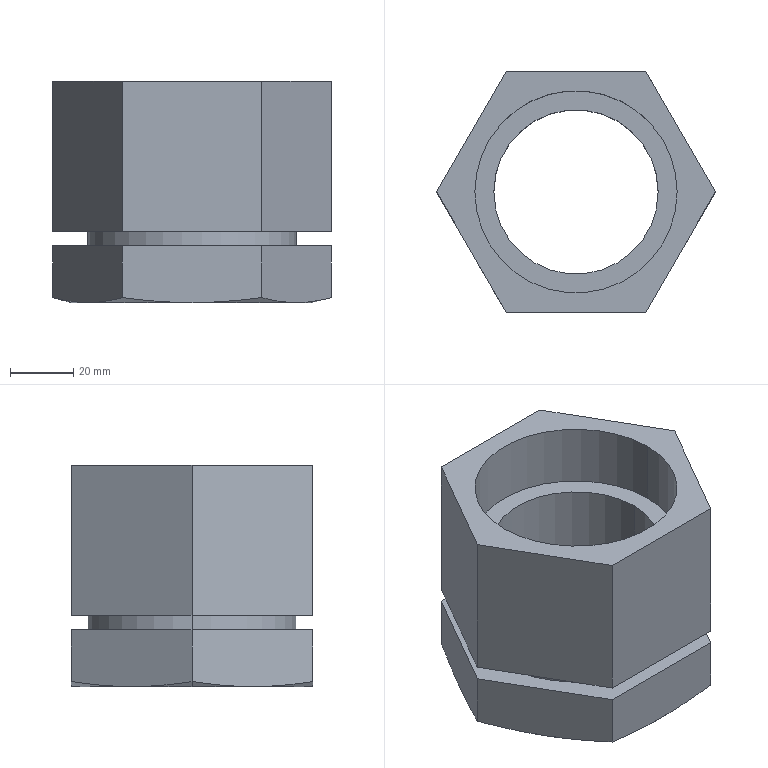Part | NX | features BREP 1 | 1 solid | 30 faces | box 88.25 x 76.427 x 70 mm | volume 175970 mm3 | plane 17 | cone 7 | cylinder 6 | commonest cylinder face diameters 52 x2 64 x2 66 x2
STEP:
#1=CARTESIAN_POINT('',(-33.,0.,22.5));
#2=VERTEX_POINT('',#1);
#3=CARTESIAN_POINT('',(33.,0.,22.5));
#4=VERTEX_POINT('',#3);
#5=CARTESIAN_POINT('',(0.,0.,22.5));
#6=DIRECTION('',(0.,0.,-1.));
#7=DIRECTION('',(-1.,0.,0.));
#8=AXIS2_PLACEMENT_3D('',#5,#6,#7);
#9=CIRCLE('',#8,33.);
#10=EDGE_CURVE('',#2,#4,#9,.T.);
#11=ORIENTED_EDGE('',*,*,#10,.T.);
#12=CARTESIAN_POINT('',(33.,0.,18.));
#13=VERTEX_POINT('',#12);
#14=CARTESIAN_POINT('',(33.,0.,0.));
#15=DIRECTION('',(0.,0.,-1.));
#16=VECTOR('',#15,1000.);
#17=LINE('',#14,#16);
#18=EDGE_CURVE('',#13,#4,#17,.F.);
#19=ORIENTED_EDGE('',*,*,#18,.F.);
#20=CARTESIAN_POINT('',(-33.,0.,18.));
#21=VERTEX_POINT('',#20);
#22=CARTESIAN_POINT('',(0.,0.,18.));
#23=DIRECTION('',(0.,0.,-1.));
#24=DIRECTION('',(-1.,0.,0.));
#25=AXIS2_PLACEMENT_3D('',#22,#23,#24);
#26=CIRCLE('',#25,33.);
#27=EDGE_CURVE('',#21,#13,#26,.T.);
#28=ORIENTED_EDGE('',*,*,#27,.F.);
#29=CARTESIAN_POINT('',(-33.,0.,0.));
#30=DIRECTION('',(0.,0.,-1.));
#31=VECTOR('',#30,1000.);
#32=LINE('',#29,#31);
#33=EDGE_CURVE('',#21,#2,#32,.F.);
#34=ORIENTED_EDGE('',*,*,#33,.T.);
#35=EDGE_LOOP('',(#11,#19,#28,#34));
#36=FACE_BOUND('',#35,.T.);
#37=CARTESIAN_POINT('',(0.,0.,0.));
#38=DIRECTION('',(0.,0.,-1.));
#39=DIRECTION('',(1.,0.,0.));
#40=AXIS2_PLACEMENT_3D('',#37,#38,#39);
#41=CYLINDRICAL_SURFACE('',#40,33.);
#42=ADVANCED_FACE('',(#36),#41,.T.);
#43=CARTESIAN_POINT('',(-32.,0.,70.));
#44=VERTEX_POINT('',#43);
#45=CARTESIAN_POINT('',(32.,0.,70.));
#46=VERTEX_POINT('',#45);
#47=CARTESIAN_POINT('',(0.,0.,70.));
#48=DIRECTION('',(0.,0.,1.));
#49=DIRECTION('',(1.,0.,0.));
#50=AXIS2_PLACEMENT_3D('',#47,#48,#49);
#51=CIRCLE('',#50,32.);
#52=EDGE_CURVE('',#44,#46,#51,.T.);
#53=ORIENTED_EDGE('',*,*,#52,.T.);
#54=CARTESIAN_POINT('',(32.,0.,50.));
#55=VERTEX_POINT('',#54);
#56=CARTESIAN_POINT('',(32.,0.,70.));
#57=DIRECTION('',(0.,0.,-1.));
#58=VECTOR('',#57,1000.);
#59=LINE('',#56,#58);
#60=EDGE_CURVE('',#55,#46,#59,.F.);
#61=ORIENTED_EDGE('',*,*,#60,.F.);
#62=CARTESIAN_POINT('',(-32.,0.,50.));
#63=VERTEX_POINT('',#62);
#64=CARTESIAN_POINT('',(0.,0.,50.));
#65=DIRECTION('',(0.,0.,1.));
#66=DIRECTION('',(1.,0.,0.));
#67=AXIS2_PLACEMENT_3D('',#64,#65,#66);
#68=CIRCLE('',#67,32.);
#69=EDGE_CURVE('',#63,#55,#68,.T.);
#70=ORIENTED_EDGE('',*,*,#69,.F.);
#71=CARTESIAN_POINT('',(-32.,0.,70.));
#72=DIRECTION('',(0.,0.,-1.));
#73=VECTOR('',#72,1000.);
#74=LINE('',#71,#73);
#75=EDGE_CURVE('',#63,#44,#74,.F.);
#76=ORIENTED_EDGE('',*,*,#75,.T.);
#77=EDGE_LOOP('',(#53,#61,#70,#76));
#78=FACE_BOUND('',#77,.T.);
#79=CARTESIAN_POINT('',(0.,0.,70.));
#80=DIRECTION('',(0.,0.,-1.));
#81=DIRECTION('',(1.,0.,0.));
#82=AXIS2_PLACEMENT_3D('',#79,#80,#81);
#83=CYLINDRICAL_SURFACE('',#82,32.);
#84=ADVANCED_FACE('',(#78),#83,.F.);
#85=CARTESIAN_POINT('',(-38.213,0.,0.));
#86=VERTEX_POINT('',#85);
#87=CARTESIAN_POINT('',(-33.094,19.107,0.));
#88=VERTEX_POINT('',#87);
#89=CARTESIAN_POINT('',(0.,0.,0.));
#90=DIRECTION('',(0.,0.,-1.));
#91=DIRECTION('',(-1.,0.,0.));
#92=AXIS2_PLACEMENT_3D('',#89,#90,#91);
#93=CIRCLE('',#92,38.213);
#94=EDGE_CURVE('',#86,#88,#93,.T.);
#95=ORIENTED_EDGE('',*,*,#94,.F.);
#96=CARTESIAN_POINT('',(-44.125,0.,1.584));
#97=VERTEX_POINT('',#96);
#98=CARTESIAN_POINT('',(-38.213,0.,0.));
#99=DIRECTION('',(-0.9659,0.,0.2588));
#100=VECTOR('',#99,1000.);
#101=LINE('',#98,#100);
#102=EDGE_CURVE('',#86,#97,#101,.T.);
#103=ORIENTED_EDGE('',*,*,#102,.T.);
#104=CARTESIAN_POINT('',(-44.125,0.,1.584));
#105=CARTESIAN_POINT('',(-40.464,6.341,0.6031));
#106=CARTESIAN_POINT('',(-36.79,12.705,0.));
#107=CARTESIAN_POINT('',(-33.094,19.107,0.));
#108=B_SPLINE_CURVE_WITH_KNOTS('',3,(#104,#105,#106,#107),.UNSPECIFIED.,.F.,.F.,(4,4),(0.,0.02212),.UNSPECIFIED.);
#109=EDGE_CURVE('',#97,#88,#108,.T.);
#110=ORIENTED_EDGE('',*,*,#109,.T.);
#111=EDGE_LOOP('',(#95,#103,#110));
#112=FACE_BOUND('',#111,.T.);
#113=CARTESIAN_POINT('',(0.,0.,0.));
#114=DIRECTION('',(0.,0.,1.));
#115=DIRECTION('',(1.,0.,0.));
#116=AXIS2_PLACEMENT_3D('',#113,#114,#115);
#117=CONICAL_SURFACE('',#116,38.213,1.309);
#118=ADVANCED_FACE('',(#112),#117,.T.);
#119=CARTESIAN_POINT('',(-26.,0.,50.));
#120=VERTEX_POINT('',#119);
#121=CARTESIAN_POINT('',(26.,0.,50.));
#122=VERTEX_POINT('',#121);
#123=CARTESIAN_POINT('',(0.,0.,50.));
#124=DIRECTION('',(0.,0.,1.));
#125=DIRECTION('',(1.,0.,0.));
#126=AXIS2_PLACEMENT_3D('',#123,#124,#125);
#127=CIRCLE('',#126,26.);
#128=EDGE_CURVE('',#120,#122,#127,.T.);
#129=ORIENTED_EDGE('',*,*,#128,.T.);
#130=CARTESIAN_POINT('',(26.,0.,0.));
#131=VERTEX_POINT('',#130);
#132=CARTESIAN_POINT('',(26.,0.,50.));
#133=DIRECTION('',(0.,0.,-1.));
#134=VECTOR('',#133,1000.);
#135=LINE('',#132,#134);
#136=EDGE_CURVE('',#131,#122,#135,.F.);
#137=ORIENTED_EDGE('',*,*,#136,.F.);
#138=CARTESIAN_POINT('',(-26.,0.,0.));
#139=VERTEX_POINT('',#138);
#140=CARTESIAN_POINT('',(0.,0.,0.));
#141=DIRECTION('',(0.,0.,1.));
#142=DIRECTION('',(1.,0.,0.));
#143=AXIS2_PLACEMENT_3D('',#140,#141,#142);
#144=CIRCLE('',#143,26.);
#145=EDGE_CURVE('',#139,#131,#144,.T.);
#146=ORIENTED_EDGE('',*,*,#145,.F.);
#147=CARTESIAN_POINT('',(-26.,0.,50.));
#148=DIRECTION('',(0.,0.,-1.));
#149=VECTOR('',#148,1000.);
#150=LINE('',#147,#149);
#151=EDGE_CURVE('',#139,#120,#150,.F.);
#152=ORIENTED_EDGE('',*,*,#151,.T.);
#153=EDGE_LOOP('',(#129,#137,#146,#152));
#154=FACE_BOUND('',#153,.T.);
#155=CARTESIAN_POINT('',(0.,0.,50.));
#156=DIRECTION('',(0.,0.,-1.));
#157=DIRECTION('',(1.,0.,0.));
#158=AXIS2_PLACEMENT_3D('',#155,#156,#157);
#159=CYLINDRICAL_SURFACE('',#158,26.);
#160=ADVANCED_FACE('',(#154),#159,.F.);
#161=CARTESIAN_POINT('',(44.125,0.,70.));
#162=VERTEX_POINT('',#161);
#163=CARTESIAN_POINT('',(44.125,0.,22.5));
#164=VERTEX_POINT('',#163);
#165=CARTESIAN_POINT('',(44.125,0.,50.));
#166=DIRECTION('',(0.,0.,-1.));
#167=VECTOR('',#166,1000.);
#168=LINE('',#165,#167);
#169=EDGE_CURVE('',#162,#164,#168,.T.);
#170=ORIENTED_EDGE('',*,*,#169,.T.);
#171=CARTESIAN_POINT('',(22.062,38.213,22.5));
#172=VERTEX_POINT('',#171);
#173=CARTESIAN_POINT('',(44.125,0.,22.5));
#174=DIRECTION('',(-0.5,0.866,0.));
#175=VECTOR('',#174,1000.);
#176=LINE('',#173,#175);
#177=EDGE_CURVE('',#164,#172,#176,.T.);
#178=ORIENTED_EDGE('',*,*,#177,.T.);
#179=CARTESIAN_POINT('',(22.062,38.213,70.));
#180=VERTEX_POINT('',#179);
#181=CARTESIAN_POINT('',(22.062,38.213,50.));
#182=DIRECTION('',(0.,0.,-1.));
#183=VECTOR('',#182,1000.);
#184=LINE('',#181,#183);
#185=EDGE_CURVE('',#180,#172,#184,.T.);
#186=ORIENTED_EDGE('',*,*,#185,.F.);
#187=CARTESIAN_POINT('',(44.125,0.,70.));
#188=DIRECTION('',(-0.5,0.866,0.));
#189=VECTOR('',#188,1000.);
#190=LINE('',#187,#189);
#191=EDGE_CURVE('',#162,#180,#190,.T.);
#192=ORIENTED_EDGE('',*,*,#191,.F.);
#193=EDGE_LOOP('',(#170,#178,#186,#192));
#194=FACE_BOUND('',#193,.T.);
#195=CARTESIAN_POINT('',(44.125,0.,50.));
#196=DIRECTION('',(-0.866,-0.5,0.));
#197=DIRECTION('',(-0.5,0.866,0.));
#198=AXIS2_PLACEMENT_3D('',#195,#196,#197);
#199=PLANE('',#198);
#200=ADVANCED_FACE('',(#194),#199,.F.);
#201=ORIENTED_EDGE('',*,*,#185,.T.);
#202=CARTESIAN_POINT('',(-22.062,38.213,22.5));
#203=VERTEX_POINT('',#202);
#204=CARTESIAN_POINT('',(22.062,38.213,22.5));
#205=DIRECTION('',(-1.,0.,0.));
#206=VECTOR('',#205,1000.);
#207=LINE('',#204,#206);
#208=EDGE_CURVE('',#172,#203,#207,.T.);
#209=ORIENTED_EDGE('',*,*,#208,.T.);
#210=CARTESIAN_POINT('',(-22.062,38.213,70.));
#211=VERTEX_POINT('',#210);
#212=CARTESIAN_POINT('',(-22.062,38.213,50.));
#213=DIRECTION('',(0.,0.,-1.));
#214=VECTOR('',#213,1000.);
#215=LINE('',#212,#214);
#216=EDGE_CURVE('',#211,#203,#215,.T.);
#217=ORIENTED_EDGE('',*,*,#216,.F.);
#218=CARTESIAN_POINT('',(22.062,38.213,70.));
#219=DIRECTION('',(-1.,0.,0.));
#220=VECTOR('',#219,1000.);
#221=LINE('',#218,#220);
#222=EDGE_CURVE('',#180,#211,#221,.T.);
#223=ORIENTED_EDGE('',*,*,#222,.F.);
#224=EDGE_LOOP('',(#201,#209,#217,#223));
#225=FACE_BOUND('',#224,.T.);
#226=CARTESIAN_POINT('',(22.062,38.213,50.));
#227=DIRECTION('',(0.,-1.,0.));
#228=DIRECTION('',(-1.,0.,0.));
#229=AXIS2_PLACEMENT_3D('',#226,#227,#228);
#230=PLANE('',#229);
#231=ADVANCED_FACE('',(#225),#230,.F.);
#232=ORIENTED_EDGE('',*,*,#216,.T.);
#233=CARTESIAN_POINT('',(-44.125,0.,22.5));
#234=VERTEX_POINT('',#233);
#235=CARTESIAN_POINT('',(-22.062,38.213,22.5));
#236=DIRECTION('',(-0.5,-0.866,0.));
#237=VECTOR('',#236,1000.);
#238=LINE('',#235,#237);
#239=EDGE_CURVE('',#203,#234,#238,.T.);
#240=ORIENTED_EDGE('',*,*,#239,.T.);
#241=CARTESIAN_POINT('',(-44.125,0.,70.));
#242=VERTEX_POINT('',#241);
#243=CARTESIAN_POINT('',(-44.125,0.,50.));
#244=DIRECTION('',(0.,0.,-1.));
#245=VECTOR('',#244,1000.);
#246=LINE('',#243,#245);
#247=EDGE_CURVE('',#242,#234,#246,.T.);
#248=ORIENTED_EDGE('',*,*,#247,.F.);
#249=CARTESIAN_POINT('',(-22.062,38.213,70.));
#250=DIRECTION('',(-0.5,-0.866,0.));
#251=VECTOR('',#250,1000.);
#252=LINE('',#249,#251);
#253=EDGE_CURVE('',#211,#242,#252,.T.);
#254=ORIENTED_EDGE('',*,*,#253,.F.);
#255=EDGE_LOOP('',(#232,#240,#248,#254));
#256=FACE_BOUND('',#255,.T.);
#257=CARTESIAN_POINT('',(-22.062,38.213,50.));
#258=DIRECTION('',(0.866,-0.5,0.));
#259=DIRECTION('',(-0.5,-0.866,0.));
#260=AXIS2_PLACEMENT_3D('',#257,#258,#259);
#261=PLANE('',#260);
#262=ADVANCED_FACE('',(#256),#261,.F.);
#263=ORIENTED_EDGE('',*,*,#247,.T.);
#264=CARTESIAN_POINT('',(-22.062,-38.213,22.5));
#265=VERTEX_POINT('',#264);
#266=CARTESIAN_POINT('',(-44.125,0.,22.5));
#267=DIRECTION('',(0.5,-0.866,0.));
#268=VECTOR('',#267,1000.);
#269=LINE('',#266,#268);
#270=EDGE_CURVE('',#234,#265,#269,.T.);
#271=ORIENTED_EDGE('',*,*,#270,.T.);
#272=CARTESIAN_POINT('',(-22.062,-38.213,70.));
#273=VERTEX_POINT('',#272);
#274=CARTESIAN_POINT('',(-22.062,-38.213,50.));
#275=DIRECTION('',(0.,0.,-1.));
#276=VECTOR('',#275,1000.);
#277=LINE('',#274,#276);
#278=EDGE_CURVE('',#273,#265,#277,.T.);
#279=ORIENTED_EDGE('',*,*,#278,.F.);
#280=CARTESIAN_POINT('',(-44.125,0.,70.));
#281=DIRECTION('',(0.5,-0.866,0.));
#282=VECTOR('',#281,1000.);
#283=LINE('',#280,#282);
#284=EDGE_CURVE('',#242,#273,#283,.T.);
#285=ORIENTED_EDGE('',*,*,#284,.F.);
#286=EDGE_LOOP('',(#263,#271,#279,#285));
#287=FACE_BOUND('',#286,.T.);
#288=CARTESIAN_POINT('',(-44.125,0.,50.));
#289=DIRECTION('',(0.866,0.5,0.));
#290=DIRECTION('',(0.5,-0.866,0.));
#291=AXIS2_PLACEMENT_3D('',#288,#289,#290);
#292=PLANE('',#291);
#293=ADVANCED_FACE('',(#287),#292,.F.);
#294=ORIENTED_EDGE('',*,*,#278,.T.);
#295=CARTESIAN_POINT('',(22.062,-38.213,22.5));
#296=VERTEX_POINT('',#295);
#297=CARTESIAN_POINT('',(-22.062,-38.213,22.5));
#298=DIRECTION('',(1.,0.,0.));
#299=VECTOR('',#298,1000.);
#300=LINE('',#297,#299);
#301=EDGE_CURVE('',#265,#296,#300,.T.);
#302=ORIENTED_EDGE('',*,*,#301,.T.);
#303=CARTESIAN_POINT('',(22.062,-38.213,70.));
#304=VERTEX_POINT('',#303);
#305=CARTESIAN_POINT('',(22.062,-38.213,50.));
#306=DIRECTION('',(0.,0.,-1.));
#307=VECTOR('',#306,1000.);
#308=LINE('',#305,#307);
#309=EDGE_CURVE('',#304,#296,#308,.T.);
#310=ORIENTED_EDGE('',*,*,#309,.F.);
#311=CARTESIAN_POINT('',(-22.062,-38.213,70.));
#312=DIRECTION('',(1.,0.,0.));
#313=VECTOR('',#312,1000.);
#314=LINE('',#311,#313);
#315=EDGE_CURVE('',#273,#304,#314,.T.);
#316=ORIENTED_EDGE('',*,*,#315,.F.);
#317=EDGE_LOOP('',(#294,#302,#310,#316));
#318=FACE_BOUND('',#317,.T.);
#319=CARTESIAN_POINT('',(-22.062,-38.213,50.));
#320=DIRECTION('',(0.,1.,0.));
#321=DIRECTION('',(1.,0.,0.));
#322=AXIS2_PLACEMENT_3D('',#319,#320,#321);
#323=PLANE('',#322);
#324=ADVANCED_FACE('',(#318),#323,.F.);
#325=ORIENTED_EDGE('',*,*,#309,.T.);
#326=CARTESIAN_POINT('',(22.062,-38.213,22.5));
#327=DIRECTION('',(0.5,0.866,0.));
#328=VECTOR('',#327,1000.);
#329=LINE('',#326,#328);
#330=EDGE_CURVE('',#296,#164,#329,.T.);
#331=ORIENTED_EDGE('',*,*,#330,.T.);
#332=ORIENTED_EDGE('',*,*,#169,.F.);
#333=CARTESIAN_POINT('',(22.062,-38.213,70.));
#334=DIRECTION('',(0.5,0.866,0.));
#335=VECTOR('',#334,1000.);
#336=LINE('',#333,#335);
#337=EDGE_CURVE('',#304,#162,#336,.T.);
#338=ORIENTED_EDGE('',*,*,#337,.F.);
#339=EDGE_LOOP('',(#325,#331,#332,#338));
#340=FACE_BOUND('',#339,.T.);
#341=CARTESIAN_POINT('',(22.062,-38.213,50.));
#342=DIRECTION('',(-0.866,0.5,0.));
#343=DIRECTION('',(0.5,0.866,0.));
#344=AXIS2_PLACEMENT_3D('',#341,#342,#343);
#345=PLANE('',#344);
#346=ADVANCED_FACE('',(#340),#345,.F.);
#347=ORIENTED_EDGE('',*,*,#145,.T.);
#348=CARTESIAN_POINT('',(0.,0.,0.));
#349=DIRECTION('',(0.,0.,1.));
#350=DIRECTION('',(1.,0.,0.));
#351=AXIS2_PLACEMENT_3D('',#348,#349,#350);
#352=CIRCLE('',#351,26.);
#353=EDGE_CURVE('',#131,#139,#352,.T.);
#354=ORIENTED_EDGE('',*,*,#353,.T.);
#355=EDGE_LOOP('',(#347,#354));
#356=FACE_BOUND('',#355,.T.);
#357=CARTESIAN_POINT('',(-33.094,-19.107,0.));
#358=VERTEX_POINT('',#357);
#359=CARTESIAN_POINT('',(0.,0.,0.));
#360=DIRECTION('',(0.,0.,-1.));
#361=DIRECTION('',(-1.,0.,0.));
#362=AXIS2_PLACEMENT_3D('',#359,#360,#361);
#363=CIRCLE('',#362,38.213);
#364=EDGE_CURVE('',#358,#86,#363,.T.);
#365=ORIENTED_EDGE('',*,*,#364,.T.);
#366=ORIENTED_EDGE('',*,*,#94,.T.);
#367=CARTESIAN_POINT('',(0.,38.213,0.));
#368=VERTEX_POINT('',#367);
#369=CARTESIAN_POINT('',(0.,0.,0.));
#370=DIRECTION('',(0.,0.,-1.));
#371=DIRECTION('',(-1.,0.,0.));
#372=AXIS2_PLACEMENT_3D('',#369,#370,#371);
#373=CIRCLE('',#372,38.213);
#374=EDGE_CURVE('',#88,#368,#373,.T.);
#375=ORIENTED_EDGE('',*,*,#374,.T.);
#376=CARTESIAN_POINT('',(33.094,19.107,0.));
#377=VERTEX_POINT('',#376);
#378=CARTESIAN_POINT('',(0.,0.,0.));
#379=DIRECTION('',(0.,0.,-1.));
#380=DIRECTION('',(-1.,0.,0.));
#381=AXIS2_PLACEMENT_3D('',#378,#379,#380);
#382=CIRCLE('',#381,38.213);
#383=EDGE_CURVE('',#368,#377,#382,.T.);
#384=ORIENTED_EDGE('',*,*,#383,.T.);
#385=CARTESIAN_POINT('',(33.094,-19.107,0.));
#386=VERTEX_POINT('',#385);
#387=CARTESIAN_POINT('',(0.,0.,0.));
#388=DIRECTION('',(0.,0.,-1.));
#389=DIRECTION('',(-1.,0.,0.));
#390=AXIS2_PLACEMENT_3D('',#387,#388,#389);
#391=CIRCLE('',#390,38.213);
#392=EDGE_CURVE('',#377,#386,#391,.T.);
#393=ORIENTED_EDGE('',*,*,#392,.T.);
#394=CARTESIAN_POINT('',(0.,-38.213,0.));
#395=VERTEX_POINT('',#394);
#396=CARTESIAN_POINT('',(0.,0.,0.));
#397=DIRECTION('',(0.,0.,-1.));
#398=DIRECTION('',(-1.,0.,0.));
#399=AXIS2_PLACEMENT_3D('',#396,#397,#398);
#400=CIRCLE('',#399,38.213);
#401=EDGE_CURVE('',#386,#395,#400,.T.);
#402=ORIENTED_EDGE('',*,*,#401,.T.);
#403=CARTESIAN_POINT('',(0.,0.,0.));
#404=DIRECTION('',(0.,0.,-1.));
#405=DIRECTION('',(-1.,0.,0.));
#406=AXIS2_PLACEMENT_3D('',#403,#404,#405);
#407=CIRCLE('',#406,38.213);
#408=EDGE_CURVE('',#395,#358,#407,.T.);
#409=ORIENTED_EDGE('',*,*,#408,.T.);
#410=EDGE_LOOP('',(#365,#366,#375,#384,#393,#402,#409));
#411=FACE_BOUND('',#410,.T.);
#412=CARTESIAN_POINT('',(66.188,-38.213,0.));
#413=DIRECTION('',(0.,0.,-1.));
#414=DIRECTION('',(1.,0.,0.));
#415=AXIS2_PLACEMENT_3D('',#412,#413,#414);
#416=PLANE('',#415);
#417=ADVANCED_FACE('',(#356,#411),#416,.T.);
#418=CARTESIAN_POINT('',(22.062,38.213,18.));
#419=VERTEX_POINT('',#418);
#420=CARTESIAN_POINT('',(22.062,38.213,1.584));
#421=VERTEX_POINT('',#420);
#422=CARTESIAN_POINT('',(22.062,38.213,50.));
#423=DIRECTION('',(0.,0.,-1.));
#424=VECTOR('',#423,1000.);
#425=LINE('',#422,#424);
#426=EDGE_CURVE('',#419,#421,#425,.T.);
#427=ORIENTED_EDGE('',*,*,#426,.F.);
#428=CARTESIAN_POINT('',(44.125,0.,18.));
#429=VERTEX_POINT('',#428);
#430=CARTESIAN_POINT('',(44.125,0.,18.));
#431=DIRECTION('',(0.5,-0.866,0.));
#432=VECTOR('',#431,1000.);
#433=LINE('',#430,#432);
#434=EDGE_CURVE('',#419,#429,#433,.T.);
#435=ORIENTED_EDGE('',*,*,#434,.T.);
#436=CARTESIAN_POINT('',(44.125,0.,1.584));
#437=VERTEX_POINT('',#436);
#438=CARTESIAN_POINT('',(44.125,0.,50.));
#439=DIRECTION('',(0.,0.,-1.));
#440=VECTOR('',#439,1000.);
#441=LINE('',#438,#440);
#442=EDGE_CURVE('',#429,#437,#441,.T.);
#443=ORIENTED_EDGE('',*,*,#442,.T.);
#444=CARTESIAN_POINT('',(33.094,19.107,0.));
#445=CARTESIAN_POINT('',(36.79,12.705,0.));
#446=CARTESIAN_POINT('',(40.464,6.341,0.6031));
#447=CARTESIAN_POINT('',(44.125,0.,1.584));
#448=B_SPLINE_CURVE_WITH_KNOTS('',3,(#444,#445,#446,#447),.UNSPECIFIED.,.F.,.F.,(4,4),(0.,0.02212),.UNSPECIFIED.);
#449=EDGE_CURVE('',#377,#437,#448,.T.);
#450=ORIENTED_EDGE('',*,*,#449,.F.);
#451=CARTESIAN_POINT('',(22.062,38.213,1.584));
#452=CARTESIAN_POINT('',(25.723,31.873,0.6031));
#453=CARTESIAN_POINT('',(29.398,25.508,0.));
#454=CARTESIAN_POINT('',(33.094,19.107,0.));
#455=B_SPLINE_CURVE_WITH_KNOTS('',3,(#451,#452,#453,#454),.UNSPECIFIED.,.F.,.F.,(4,4),(0.,0.02212),.UNSPECIFIED.);
#456=EDGE_CURVE('',#421,#377,#455,.T.);
#457=ORIENTED_EDGE('',*,*,#456,.F.);
#458=EDGE_LOOP('',(#427,#435,#443,#450,#457));
#459=FACE_BOUND('',#458,.T.);
#460=CARTESIAN_POINT('',(44.125,0.,50.));
#461=DIRECTION('',(-0.866,-0.5,0.));
#462=DIRECTION('',(-0.5,0.866,0.));
#463=AXIS2_PLACEMENT_3D('',#460,#461,#462);
#464=PLANE('',#463);
#465=ADVANCED_FACE('',(#459),#464,.F.);
#466=CARTESIAN_POINT('',(-22.062,38.213,18.));
#467=VERTEX_POINT('',#466);
#468=CARTESIAN_POINT('',(-22.062,38.213,1.584));
#469=VERTEX_POINT('',#468);
#470=CARTESIAN_POINT('',(-22.062,38.213,50.));
#471=DIRECTION('',(0.,0.,-1.));
#472=VECTOR('',#471,1000.);
#473=LINE('',#470,#472);
#474=EDGE_CURVE('',#467,#469,#473,.T.);
#475=ORIENTED_EDGE('',*,*,#474,.F.);
#476=CARTESIAN_POINT('',(22.062,38.213,18.));
#477=DIRECTION('',(1.,0.,0.));
#478=VECTOR('',#477,1000.);
#479=LINE('',#476,#478);
#480=EDGE_CURVE('',#467,#419,#479,.T.);
#481=ORIENTED_EDGE('',*,*,#480,.T.);
#482=ORIENTED_EDGE('',*,*,#426,.T.);
#483=CARTESIAN_POINT('',(0.,38.213,0.));
#484=CARTESIAN_POINT('',(7.392,38.213,0.));
#485=CARTESIAN_POINT('',(14.741,38.213,0.6031));
#486=CARTESIAN_POINT('',(22.062,38.213,1.584));
#487=B_SPLINE_CURVE_WITH_KNOTS('',3,(#483,#484,#485,#486),.UNSPECIFIED.,.F.,.F.,(4,4),(0.,0.02212),.UNSPECIFIED.);
#488=EDGE_CURVE('',#368,#421,#487,.T.);
#489=ORIENTED_EDGE('',*,*,#488,.F.);
#490=CARTESIAN_POINT('',(-22.062,38.213,1.584));
#491=CARTESIAN_POINT('',(-14.741,38.213,0.6031));
#492=CARTESIAN_POINT('',(-7.392,38.213,0.));
#493=CARTESIAN_POINT('',(0.,38.213,0.));
#494=B_SPLINE_CURVE_WITH_KNOTS('',3,(#490,#491,#492,#493),.UNSPECIFIED.,.F.,.F.,(4,4),(0.,0.02212),.UNSPECIFIED.);
#495=EDGE_CURVE('',#469,#368,#494,.T.);
#496=ORIENTED_EDGE('',*,*,#495,.F.);
#497=EDGE_LOOP('',(#475,#481,#482,#489,#496));
#498=FACE_BOUND('',#497,.T.);
#499=CARTESIAN_POINT('',(22.062,38.213,50.));
#500=DIRECTION('',(0.,-1.,0.));
#501=DIRECTION('',(-1.,0.,0.));
#502=AXIS2_PLACEMENT_3D('',#499,#500,#501);
#503=PLANE('',#502);
#504=ADVANCED_FACE('',(#498),#503,.F.);
#505=CARTESIAN_POINT('',(-44.125,0.,18.));
#506=VERTEX_POINT('',#505);
#507=CARTESIAN_POINT('',(-44.125,0.,50.));
#508=DIRECTION('',(0.,0.,-1.));
#509=VECTOR('',#508,1000.);
#510=LINE('',#507,#509);
#511=EDGE_CURVE('',#506,#97,#510,.T.);
#512=ORIENTED_EDGE('',*,*,#511,.F.);
#513=CARTESIAN_POINT('',(-22.062,38.213,18.));
#514=DIRECTION('',(0.5,0.866,0.));
#515=VECTOR('',#514,1000.);
#516=LINE('',#513,#515);
#517=EDGE_CURVE('',#506,#467,#516,.T.);
#518=ORIENTED_EDGE('',*,*,#517,.T.);
#519=ORIENTED_EDGE('',*,*,#474,.T.);
#520=CARTESIAN_POINT('',(-33.094,19.107,0.));
#521=CARTESIAN_POINT('',(-29.398,25.508,0.));
#522=CARTESIAN_POINT('',(-25.723,31.873,0.6031));
#523=CARTESIAN_POINT('',(-22.062,38.213,1.584));
#524=B_SPLINE_CURVE_WITH_KNOTS('',3,(#520,#521,#522,#523),.UNSPECIFIED.,.F.,.F.,(4,4),(0.,0.02212),.UNSPECIFIED.);
#525=EDGE_CURVE('',#88,#469,#524,.T.);
#526=ORIENTED_EDGE('',*,*,#525,.F.);
#527=ORIENTED_EDGE('',*,*,#109,.F.);
#528=EDGE_LOOP('',(#512,#518,#519,#526,#527));
#529=FACE_BOUND('',#528,.T.);
#530=CARTESIAN_POINT('',(-22.062,38.213,50.));
#531=DIRECTION('',(0.866,-0.5,0.));
#532=DIRECTION('',(-0.5,-0.866,0.));
#533=AXIS2_PLACEMENT_3D('',#530,#531,#532);
#534=PLANE('',#533);
#535=ADVANCED_FACE('',(#529),#534,.F.);
#536=CARTESIAN_POINT('',(-22.062,-38.213,18.));
#537=VERTEX_POINT('',#536);
#538=CARTESIAN_POINT('',(-22.062,-38.213,1.584));
#539=VERTEX_POINT('',#538);
#540=CARTESIAN_POINT('',(-22.062,-38.213,50.));
#541=DIRECTION('',(0.,0.,-1.));
#542=VECTOR('',#541,1000.);
#543=LINE('',#540,#542);
#544=EDGE_CURVE('',#537,#539,#543,.T.);
#545=ORIENTED_EDGE('',*,*,#544,.F.);
#546=CARTESIAN_POINT('',(-44.125,0.,18.));
#547=DIRECTION('',(-0.5,0.866,0.));
#548=VECTOR('',#547,1000.);
#549=LINE('',#546,#548);
#550=EDGE_CURVE('',#537,#506,#549,.T.);
#551=ORIENTED_EDGE('',*,*,#550,.T.);
#552=ORIENTED_EDGE('',*,*,#511,.T.);
#553=CARTESIAN_POINT('',(-33.094,-19.107,0.));
#554=CARTESIAN_POINT('',(-36.79,-12.705,0.));
#555=CARTESIAN_POINT('',(-40.464,-6.341,0.6031));
#556=CARTESIAN_POINT('',(-44.125,0.,1.584));
#557=B_SPLINE_CURVE_WITH_KNOTS('',3,(#553,#554,#555,#556),.UNSPECIFIED.,.F.,.F.,(4,4),(0.,0.02212),.UNSPECIFIED.);
#558=EDGE_CURVE('',#358,#97,#557,.T.);
#559=ORIENTED_EDGE('',*,*,#558,.F.);
#560=CARTESIAN_POINT('',(-22.062,-38.213,1.584));
#561=CARTESIAN_POINT('',(-25.723,-31.873,0.6031));
#562=CARTESIAN_POINT('',(-29.398,-25.508,0.));
#563=CARTESIAN_POINT('',(-33.094,-19.107,0.));
#564=B_SPLINE_CURVE_WITH_KNOTS('',3,(#560,#561,#562,#563),.UNSPECIFIED.,.F.,.F.,(4,4),(0.,0.02212),.UNSPECIFIED.);
#565=EDGE_CURVE('',#539,#358,#564,.T.);
#566=ORIENTED_EDGE('',*,*,#565,.F.);
#567=EDGE_LOOP('',(#545,#551,#552,#559,#566));
#568=FACE_BOUND('',#567,.T.);
#569=CARTESIAN_POINT('',(-44.125,0.,50.));
#570=DIRECTION('',(0.866,0.5,0.));
#571=DIRECTION('',(0.5,-0.866,0.));
#572=AXIS2_PLACEMENT_3D('',#569,#570,#571);
#573=PLANE('',#572);
#574=ADVANCED_FACE('',(#568),#573,.F.);
#575=CARTESIAN_POINT('',(22.062,-38.213,18.));
#576=VERTEX_POINT('',#575);
#577=CARTESIAN_POINT('',(22.062,-38.213,1.584));
#578=VERTEX_POINT('',#577);
#579=CARTESIAN_POINT('',(22.062,-38.213,50.));
#580=DIRECTION('',(0.,0.,-1.));
#581=VECTOR('',#580,1000.);
#582=LINE('',#579,#581);
#583=EDGE_CURVE('',#576,#578,#582,.T.);
#584=ORIENTED_EDGE('',*,*,#583,.F.);
#585=CARTESIAN_POINT('',(-22.062,-38.213,18.));
#586=DIRECTION('',(-1.,0.,0.));
#587=VECTOR('',#586,1000.);
#588=LINE('',#585,#587);
#589=EDGE_CURVE('',#576,#537,#588,.T.);
#590=ORIENTED_EDGE('',*,*,#589,.T.);
#591=ORIENTED_EDGE('',*,*,#544,.T.);
#592=CARTESIAN_POINT('',(0.,-38.213,0.));
#593=CARTESIAN_POINT('',(-7.392,-38.213,0.));
#594=CARTESIAN_POINT('',(-14.741,-38.213,0.6031));
#595=CARTESIAN_POINT('',(-22.062,-38.213,1.584));
#596=B_SPLINE_CURVE_WITH_KNOTS('',3,(#592,#593,#594,#595),.UNSPECIFIED.,.F.,.F.,(4,4),(0.,0.02212),.UNSPECIFIED.);
#597=EDGE_CURVE('',#395,#539,#596,.T.);
#598=ORIENTED_EDGE('',*,*,#597,.F.);
#599=CARTESIAN_POINT('',(22.062,-38.213,1.584));
#600=CARTESIAN_POINT('',(14.741,-38.213,0.6031));
#601=CARTESIAN_POINT('',(7.392,-38.213,0.));
#602=CARTESIAN_POINT('',(0.,-38.213,0.));
#603=B_SPLINE_CURVE_WITH_KNOTS('',3,(#599,#600,#601,#602),.UNSPECIFIED.,.F.,.F.,(4,4),(0.,0.02212),.UNSPECIFIED.);
#604=EDGE_CURVE('',#578,#395,#603,.T.);
#605=ORIENTED_EDGE('',*,*,#604,.F.);
#606=EDGE_LOOP('',(#584,#590,#591,#598,#605));
#607=FACE_BOUND('',#606,.T.);
#608=CARTESIAN_POINT('',(-22.062,-38.213,50.));
#609=DIRECTION('',(0.,1.,0.));
#610=DIRECTION('',(1.,0.,0.));
#611=AXIS2_PLACEMENT_3D('',#608,#609,#610);
#612=PLANE('',#611);
#613=ADVANCED_FACE('',(#607),#612,.F.);
#614=ORIENTED_EDGE('',*,*,#442,.F.);
#615=CARTESIAN_POINT('',(22.062,-38.213,18.));
#616=DIRECTION('',(-0.5,-0.866,0.));
#617=VECTOR('',#616,1000.);
#618=LINE('',#615,#617);
#619=EDGE_CURVE('',#429,#576,#618,.T.);
#620=ORIENTED_EDGE('',*,*,#619,.T.);
#621=ORIENTED_EDGE('',*,*,#583,.T.);
#622=CARTESIAN_POINT('',(33.094,-19.107,0.));
#623=CARTESIAN_POINT('',(29.398,-25.508,0.));
#624=CARTESIAN_POINT('',(25.723,-31.873,0.6031));
#625=CARTESIAN_POINT('',(22.062,-38.213,1.584));
#626=B_SPLINE_CURVE_WITH_KNOTS('',3,(#622,#623,#624,#625),.UNSPECIFIED.,.F.,.F.,(4,4),(0.,0.02212),.UNSPECIFIED.);
#627=EDGE_CURVE('',#386,#578,#626,.T.);
#628=ORIENTED_EDGE('',*,*,#627,.F.);
#629=CARTESIAN_POINT('',(44.125,0.,1.584));
#630=CARTESIAN_POINT('',(40.464,-6.341,0.6031));
#631=CARTESIAN_POINT('',(36.79,-12.705,0.));
#632=CARTESIAN_POINT('',(33.094,-19.107,0.));
#633=B_SPLINE_CURVE_WITH_KNOTS('',3,(#629,#630,#631,#632),.UNSPECIFIED.,.F.,.F.,(4,4),(0.,0.02212),.UNSPECIFIED.);
#634=EDGE_CURVE('',#437,#386,#633,.T.);
#635=ORIENTED_EDGE('',*,*,#634,.F.);
#636=EDGE_LOOP('',(#614,#620,#621,#628,#635));
#637=FACE_BOUND('',#636,.T.);
#638=CARTESIAN_POINT('',(22.062,-38.213,50.));
#639=DIRECTION('',(-0.866,0.5,0.));
#640=DIRECTION('',(0.5,0.866,0.));
#641=AXIS2_PLACEMENT_3D('',#638,#639,#640);
#642=PLANE('',#641);
#643=ADVANCED_FACE('',(#637),#642,.F.);
#644=ORIENTED_EDGE('',*,*,#69,.T.);
#645=CARTESIAN_POINT('',(0.,0.,50.));
#646=DIRECTION('',(0.,0.,1.));
#647=DIRECTION('',(1.,0.,0.));
#648=AXIS2_PLACEMENT_3D('',#645,#646,#647);
#649=CIRCLE('',#648,32.);
#650=EDGE_CURVE('',#55,#63,#649,.T.);
#651=ORIENTED_EDGE('',*,*,#650,.T.);
#652=EDGE_LOOP('',(#644,#651));
#653=FACE_BOUND('',#652,.T.);
#654=ORIENTED_EDGE('',*,*,#128,.F.);
#655=CARTESIAN_POINT('',(0.,0.,50.));
#656=DIRECTION('',(0.,0.,1.));
#657=DIRECTION('',(1.,0.,0.));
#658=AXIS2_PLACEMENT_3D('',#655,#656,#657);
#659=CIRCLE('',#658,26.);
#660=EDGE_CURVE('',#122,#120,#659,.T.);
#661=ORIENTED_EDGE('',*,*,#660,.F.);
#662=EDGE_LOOP('',(#654,#661));
#663=FACE_BOUND('',#662,.T.);
#664=CARTESIAN_POINT('',(66.188,-38.213,50.));
#665=DIRECTION('',(0.,0.,-1.));
#666=DIRECTION('',(1.,0.,0.));
#667=AXIS2_PLACEMENT_3D('',#664,#665,#666);
#668=PLANE('',#667);
#669=ADVANCED_FACE('',(#653,#663),#668,.F.);
#670=ORIENTED_EDGE('',*,*,#136,.T.);
#671=ORIENTED_EDGE('',*,*,#660,.T.);
#672=ORIENTED_EDGE('',*,*,#151,.F.);
#673=ORIENTED_EDGE('',*,*,#353,.F.);
#674=EDGE_LOOP('',(#670,#671,#672,#673));
#675=FACE_BOUND('',#674,.T.);
#676=CARTESIAN_POINT('',(0.,0.,50.));
#677=DIRECTION('',(0.,0.,-1.));
#678=DIRECTION('',(1.,0.,0.));
#679=AXIS2_PLACEMENT_3D('',#676,#677,#678);
#680=CYLINDRICAL_SURFACE('',#679,26.);
#681=ADVANCED_FACE('',(#675),#680,.F.);
#682=ORIENTED_EDGE('',*,*,#604,.T.);
#683=ORIENTED_EDGE('',*,*,#401,.F.);
#684=ORIENTED_EDGE('',*,*,#627,.T.);
#685=EDGE_LOOP('',(#682,#683,#684));
#686=FACE_BOUND('',#685,.T.);
#687=CARTESIAN_POINT('',(0.,0.,0.));
#688=DIRECTION('',(0.,0.,1.));
#689=DIRECTION('',(1.,0.,0.));
#690=AXIS2_PLACEMENT_3D('',#687,#688,#689);
#691=CONICAL_SURFACE('',#690,38.213,1.309);
#692=ADVANCED_FACE('',(#686),#691,.T.);
#693=ORIENTED_EDGE('',*,*,#449,.T.);
#694=ORIENTED_EDGE('',*,*,#634,.T.);
#695=ORIENTED_EDGE('',*,*,#392,.F.);
#696=EDGE_LOOP('',(#693,#694,#695));
#697=FACE_BOUND('',#696,.T.);
#698=CARTESIAN_POINT('',(0.,0.,0.));
#699=DIRECTION('',(0.,0.,1.));
#700=DIRECTION('',(1.,0.,0.));
#701=AXIS2_PLACEMENT_3D('',#698,#699,#700);
#702=CONICAL_SURFACE('',#701,38.213,1.309);
#703=ADVANCED_FACE('',(#697),#702,.T.);
#704=ORIENTED_EDGE('',*,*,#565,.T.);
#705=ORIENTED_EDGE('',*,*,#408,.F.);
#706=ORIENTED_EDGE('',*,*,#597,.T.);
#707=EDGE_LOOP('',(#704,#705,#706));
#708=FACE_BOUND('',#707,.T.);
#709=CARTESIAN_POINT('',(0.,0.,0.));
#710=DIRECTION('',(0.,0.,1.));
#711=DIRECTION('',(1.,0.,0.));
#712=AXIS2_PLACEMENT_3D('',#709,#710,#711);
#713=CONICAL_SURFACE('',#712,38.213,1.309);
#714=ADVANCED_FACE('',(#708),#713,.T.);
#715=ORIENTED_EDGE('',*,*,#102,.F.);
#716=ORIENTED_EDGE('',*,*,#364,.F.);
#717=ORIENTED_EDGE('',*,*,#558,.T.);
#718=EDGE_LOOP('',(#715,#716,#717));
#719=FACE_BOUND('',#718,.T.);
#720=CARTESIAN_POINT('',(0.,0.,0.));
#721=DIRECTION('',(0.,0.,1.));
#722=DIRECTION('',(1.,0.,0.));
#723=AXIS2_PLACEMENT_3D('',#720,#721,#722);
#724=CONICAL_SURFACE('',#723,38.213,1.309);
#725=ADVANCED_FACE('',(#719),#724,.T.);
#726=ORIENTED_EDGE('',*,*,#525,.T.);
#727=ORIENTED_EDGE('',*,*,#495,.T.);
#728=ORIENTED_EDGE('',*,*,#374,.F.);
#729=EDGE_LOOP('',(#726,#727,#728));
#730=FACE_BOUND('',#729,.T.);
#731=CARTESIAN_POINT('',(0.,0.,0.));
#732=DIRECTION('',(0.,0.,1.));
#733=DIRECTION('',(1.,0.,0.));
#734=AXIS2_PLACEMENT_3D('',#731,#732,#733);
#735=CONICAL_SURFACE('',#734,38.213,1.309);
#736=ADVANCED_FACE('',(#730),#735,.T.);
#737=ORIENTED_EDGE('',*,*,#488,.T.);
#738=ORIENTED_EDGE('',*,*,#456,.T.);
#739=ORIENTED_EDGE('',*,*,#383,.F.);
#740=EDGE_LOOP('',(#737,#738,#739));
#741=FACE_BOUND('',#740,.T.);
#742=CARTESIAN_POINT('',(0.,0.,0.));
#743=DIRECTION('',(0.,0.,1.));
#744=DIRECTION('',(1.,0.,0.));
#745=AXIS2_PLACEMENT_3D('',#742,#743,#744);
#746=CONICAL_SURFACE('',#745,38.213,1.309);
#747=ADVANCED_FACE('',(#741),#746,.T.);
#748=ORIENTED_EDGE('',*,*,#337,.T.);
#749=ORIENTED_EDGE('',*,*,#191,.T.);
#750=ORIENTED_EDGE('',*,*,#222,.T.);
#751=ORIENTED_EDGE('',*,*,#253,.T.);
#752=ORIENTED_EDGE('',*,*,#284,.T.);
#753=ORIENTED_EDGE('',*,*,#315,.T.);
#754=EDGE_LOOP('',(#748,#749,#750,#751,#752,#753));
#755=FACE_BOUND('',#754,.T.);
#756=ORIENTED_EDGE('',*,*,#52,.F.);
#757=CARTESIAN_POINT('',(0.,0.,70.));
#758=DIRECTION('',(0.,0.,1.));
#759=DIRECTION('',(1.,0.,0.));
#760=AXIS2_PLACEMENT_3D('',#757,#758,#759);
#761=CIRCLE('',#760,32.);
#762=EDGE_CURVE('',#46,#44,#761,.T.);
#763=ORIENTED_EDGE('',*,*,#762,.F.);
#764=EDGE_LOOP('',(#756,#763));
#765=FACE_BOUND('',#764,.T.);
#766=CARTESIAN_POINT('',(66.188,38.213,70.));
#767=DIRECTION('',(0.,0.,1.));
#768=DIRECTION('',(-1.,0.,0.));
#769=AXIS2_PLACEMENT_3D('',#766,#767,#768);
#770=PLANE('',#769);
#771=ADVANCED_FACE('',(#755,#765),#770,.T.);
#772=ORIENTED_EDGE('',*,*,#60,.T.);
#773=ORIENTED_EDGE('',*,*,#762,.T.);
#774=ORIENTED_EDGE('',*,*,#75,.F.);
#775=ORIENTED_EDGE('',*,*,#650,.F.);
#776=EDGE_LOOP('',(#772,#773,#774,#775));
#777=FACE_BOUND('',#776,.T.);
#778=CARTESIAN_POINT('',(0.,0.,70.));
#779=DIRECTION('',(0.,0.,-1.));
#780=DIRECTION('',(1.,0.,0.));
#781=AXIS2_PLACEMENT_3D('',#778,#779,#780);
#782=CYLINDRICAL_SURFACE('',#781,32.);
#783=ADVANCED_FACE('',(#777),#782,.F.);
#784=ORIENTED_EDGE('',*,*,#10,.F.);
#785=CARTESIAN_POINT('',(0.,0.,22.5));
#786=DIRECTION('',(0.,0.,-1.));
#787=DIRECTION('',(-1.,0.,0.));
#788=AXIS2_PLACEMENT_3D('',#785,#786,#787);
#789=CIRCLE('',#788,33.);
#790=EDGE_CURVE('',#4,#2,#789,.T.);
#791=ORIENTED_EDGE('',*,*,#790,.F.);
#792=EDGE_LOOP('',(#784,#791));
#793=FACE_BOUND('',#792,.T.);
#794=ORIENTED_EDGE('',*,*,#330,.F.);
#795=ORIENTED_EDGE('',*,*,#301,.F.);
#796=ORIENTED_EDGE('',*,*,#270,.F.);
#797=ORIENTED_EDGE('',*,*,#239,.F.);
#798=ORIENTED_EDGE('',*,*,#208,.F.);
#799=ORIENTED_EDGE('',*,*,#177,.F.);
#800=EDGE_LOOP('',(#794,#795,#796,#797,#798,#799));
#801=FACE_BOUND('',#800,.T.);
#802=CARTESIAN_POINT('',(0.,59.386,22.5));
#803=DIRECTION('',(0.,0.,1.));
#804=DIRECTION('',(-1.,0.,0.));
#805=AXIS2_PLACEMENT_3D('',#802,#803,#804);
#806=PLANE('',#805);
#807=ADVANCED_FACE('',(#793,#801),#806,.F.);
#808=ORIENTED_EDGE('',*,*,#27,.T.);
#809=CARTESIAN_POINT('',(0.,0.,18.));
#810=DIRECTION('',(0.,0.,-1.));
#811=DIRECTION('',(-1.,0.,0.));
#812=AXIS2_PLACEMENT_3D('',#809,#810,#811);
#813=CIRCLE('',#812,33.);
#814=EDGE_CURVE('',#13,#21,#813,.T.);
#815=ORIENTED_EDGE('',*,*,#814,.T.);
#816=EDGE_LOOP('',(#808,#815));
#817=FACE_BOUND('',#816,.T.);
#818=ORIENTED_EDGE('',*,*,#480,.F.);
#819=ORIENTED_EDGE('',*,*,#517,.F.);
#820=ORIENTED_EDGE('',*,*,#550,.F.);
#821=ORIENTED_EDGE('',*,*,#589,.F.);
#822=ORIENTED_EDGE('',*,*,#619,.F.);
#823=ORIENTED_EDGE('',*,*,#434,.F.);
#824=EDGE_LOOP('',(#818,#819,#820,#821,#822,#823));
#825=FACE_BOUND('',#824,.T.);
#826=CARTESIAN_POINT('',(0.,59.386,18.));
#827=DIRECTION('',(0.,0.,-1.));
#828=DIRECTION('',(1.,0.,0.));
#829=AXIS2_PLACEMENT_3D('',#826,#827,#828);
#830=PLANE('',#829);
#831=ADVANCED_FACE('',(#817,#825),#830,.F.);
#832=ORIENTED_EDGE('',*,*,#18,.T.);
#833=ORIENTED_EDGE('',*,*,#790,.T.);
#834=ORIENTED_EDGE('',*,*,#33,.F.);
#835=ORIENTED_EDGE('',*,*,#814,.F.);
#836=EDGE_LOOP('',(#832,#833,#834,#835));
#837=FACE_BOUND('',#836,.T.);
#838=CARTESIAN_POINT('',(0.,0.,0.));
#839=DIRECTION('',(0.,0.,-1.));
#840=DIRECTION('',(1.,0.,0.));
#841=AXIS2_PLACEMENT_3D('',#838,#839,#840);
#842=CYLINDRICAL_SURFACE('',#841,33.);
#843=ADVANCED_FACE('',(#837),#842,.T.);
#844=CLOSED_SHELL('',(#42,#84,#118,#160,#200,#231,#262,#293,#324,#346,#417,#465,#504,#535,#574,#613,#643,#669,#681,#692,#703,#714,#725,#736,#747,#771,#783,#807,#831,#843));
#845=MANIFOLD_SOLID_BREP('',#844);
#846=(LENGTH_UNIT()NAMED_UNIT(*)SI_UNIT(.MILLI.,.METRE.));
#847=UNCERTAINTY_MEASURE_WITH_UNIT(LENGTH_MEASURE(0.0508),#846,'','');
#848=(NAMED_UNIT(*)PLANE_ANGLE_UNIT()SI_UNIT($,.RADIAN.));
#849=(NAMED_UNIT(*)SI_UNIT($,.STERADIAN.)SOLID_ANGLE_UNIT());
#850=(GEOMETRIC_REPRESENTATION_CONTEXT(3)GLOBAL_UNCERTAINTY_ASSIGNED_CONTEXT((#847))GLOBAL_UNIT_ASSIGNED_CONTEXT((#846,#848,#849))REPRESENTATION_CONTEXT('',''));
#851=ADVANCED_BREP_SHAPE_REPRESENTATION('',(#845),#850);